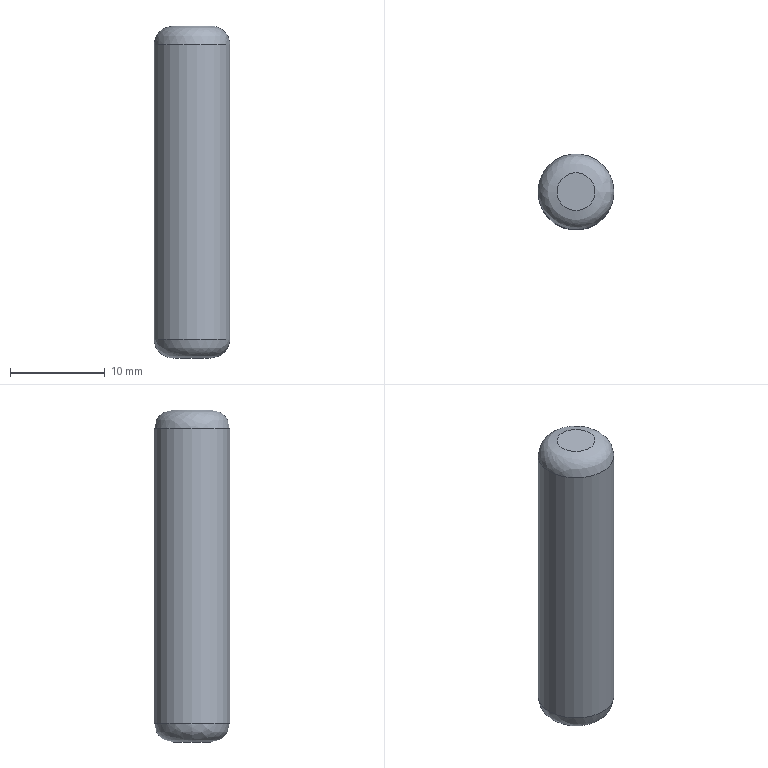Part | STEP file | Tube feed_id1706_x_t | 1 solid | 5 faces | box 8 x 8 x 35 mm | volume 1721 mm3 | plane 2 | spline 2 | cylinder 1 | commonest cylinder face diameters 8 x1
STEP:
#1=CARTESIAN_POINT('',(0.,0.,0.));
#2=DIRECTION('',(0.,0.,1.));
#3=DIRECTION('',(1.,0.,0.));
#4=AXIS2_PLACEMENT_3D('',#1,#2,#3);
#5=CARTESIAN_POINT('',(119.,82.036,-214.5));
#6=VERTEX_POINT('',#5);
#7=CARTESIAN_POINT('',(121.,82.036,-214.5));
#8=DIRECTION('',(0.,0.,-1.));
#9=DIRECTION('',(-1.,0.,0.));
#10=AXIS2_PLACEMENT_3D('',#7,#8,#9);
#11=CIRCLE('',#10,2.);
#12=CARTESIAN_POINT('',(121.,82.036,-214.5));
#13=DIRECTION('',(0.,0.,-1.));
#14=DIRECTION('',(-1.,0.,0.));
#15=AXIS2_PLACEMENT_3D('',#12,#13,#14);
#16=PLANE('',#15);
#17=CARTESIAN_POINT('',(0.,0.));
#18=DIRECTION('',(1.,0.));
#19=AXIS2_PLACEMENT_2D('',#17,#18);
#20=CIRCLE('',#19,2.);
#21=(GEOMETRIC_REPRESENTATION_CONTEXT(2)PARAMETRIC_REPRESENTATION_CONTEXT()REPRESENTATION_CONTEXT('',''));
#22=DEFINITIONAL_REPRESENTATION('',(#20),#21);
#23=PCURVE('',#16,#22);
#24=CARTESIAN_POINT('',(119.,82.036,-214.5));
#25=CARTESIAN_POINT('',(119.,86.036,-214.5));
#26=CARTESIAN_POINT('',(123.,86.036,-214.5));
#27=CARTESIAN_POINT('',(123.,82.036,-214.5));
#28=CARTESIAN_POINT('',(123.,78.036,-214.5));
#29=CARTESIAN_POINT('',(119.,78.036,-214.5));
#30=CARTESIAN_POINT('',(119.,82.036,-214.5));
#31=CARTESIAN_POINT('',(117.828,82.036,-214.5));
#32=CARTESIAN_POINT('',(117.828,88.379,-214.5));
#33=CARTESIAN_POINT('',(124.172,88.379,-214.5));
#34=CARTESIAN_POINT('',(124.172,82.036,-214.5));
#35=CARTESIAN_POINT('',(124.172,75.692,-214.5));
#36=CARTESIAN_POINT('',(117.828,75.692,-214.5));
#37=CARTESIAN_POINT('',(117.828,82.036,-214.5));
#38=CARTESIAN_POINT('',(117.,82.036,-213.672));
#39=CARTESIAN_POINT('',(117.,90.036,-213.672));
#40=CARTESIAN_POINT('',(125.,90.036,-213.672));
#41=CARTESIAN_POINT('',(125.,82.036,-213.672));
#42=CARTESIAN_POINT('',(125.,74.036,-213.672));
#43=CARTESIAN_POINT('',(117.,74.036,-213.672));
#44=CARTESIAN_POINT('',(117.,82.036,-213.672));
#45=CARTESIAN_POINT('',(117.,82.036,-212.5));
#46=CARTESIAN_POINT('',(117.,90.036,-212.5));
#47=CARTESIAN_POINT('',(125.,90.036,-212.5));
#48=CARTESIAN_POINT('',(125.,82.036,-212.5));
#49=CARTESIAN_POINT('',(125.,74.036,-212.5));
#50=CARTESIAN_POINT('',(117.,74.036,-212.5));
#51=CARTESIAN_POINT('',(117.,82.036,-212.5));
#52=(BOUNDED_SURFACE()B_SPLINE_SURFACE(3,3,((#24,#25,#26,#27,#28,#29,#30),(#31,#32,#33,#34,#35,#36,#37),(#38,#39,#40,#41,#42,#43,#44),(#45,#46,#47,#48,#49,#50,#51)),.UNSPECIFIED.,.F.,.T.,.F.)B_SPLINE_SURFACE_WITH_KNOTS((4,4),(1,3,3,3,1),(0.,1.),(-0.5,0.,0.5,1.,1.5),.UNSPECIFIED.)GEOMETRIC_REPRESENTATION_ITEM()RATIONAL_B_SPLINE_SURFACE(((1.,0.3333,0.3333,1.,0.3333,0.3333,1.),(0.8047,0.2682,0.2682,0.8047,0.2682,0.2682,0.8047),(0.8047,0.2682,0.2682,0.8047,0.2682,0.2682,0.8047),(1.,0.3333,0.3333,1.,0.3333,0.3333,1.)))REPRESENTATION_ITEM('')SURFACE());
#53=CARTESIAN_POINT('',(0.,0.));
#54=CARTESIAN_POINT('',(0.,0.02352));
#55=CARTESIAN_POINT('',(0.,0.06491));
#56=CARTESIAN_POINT('',(0.,0.1146));
#57=CARTESIAN_POINT('',(0.,0.1575));
#58=CARTESIAN_POINT('',(0.,0.196));
#59=CARTESIAN_POINT('',(0.,0.2322));
#60=CARTESIAN_POINT('',(0.,0.2678));
#61=CARTESIAN_POINT('',(0.,0.304));
#62=CARTESIAN_POINT('',(0.,0.3425));
#63=CARTESIAN_POINT('',(0.,0.3856));
#64=CARTESIAN_POINT('',(0.,0.4343));
#65=CARTESIAN_POINT('',(0.,0.5));
#66=CARTESIAN_POINT('',(0.,0.5657));
#67=CARTESIAN_POINT('',(0.,0.6144));
#68=CARTESIAN_POINT('',(0.,0.6575));
#69=CARTESIAN_POINT('',(0.,0.696));
#70=CARTESIAN_POINT('',(0.,0.7322));
#71=CARTESIAN_POINT('',(0.,0.7678));
#72=CARTESIAN_POINT('',(0.,0.804));
#73=CARTESIAN_POINT('',(0.,0.8425));
#74=CARTESIAN_POINT('',(0.,0.8854));
#75=CARTESIAN_POINT('',(0.,0.9351));
#76=CARTESIAN_POINT('',(0.,0.9765));
#77=CARTESIAN_POINT('',(0.,1.));
#78=B_SPLINE_CURVE_WITH_KNOTS('',3,(#53,#54,#55,#56,#57,#58,#59,#60,#61,#62,#63,#64,#65,#66,#67,#68,#69,#70,#71,#72,#73,#74,#75,#76,#77),.UNSPECIFIED.,.F.,.F.,(4,1,1,1,1,1,1,1,1,1,1,1,1,1,1,1,1,1,1,1,1,1,4),(0.,0.2856,0.5712,0.8568,1.142,1.428,1.714,1.999,2.285,2.57,2.856,3.142,3.427,3.713,3.998,4.284,4.57,4.855,5.141,5.426,5.712,5.998,6.283),.QUASI_UNIFORM_KNOTS.);
#79=(GEOMETRIC_REPRESENTATION_CONTEXT(2)PARAMETRIC_REPRESENTATION_CONTEXT()REPRESENTATION_CONTEXT('',''));
#80=DEFINITIONAL_REPRESENTATION('',(#78),#79);
#81=PCURVE('',#52,#80);
#82=SURFACE_CURVE('',#11,(#23,#81),.PCURVE_S1.);
#83=EDGE_CURVE('',#6,#6,#82,.T.);
#84=ORIENTED_EDGE('',*,*,#83,.T.);
#85=EDGE_LOOP('',(#84));
#86=FACE_BOUND('',#85,.T.);
#87=ADVANCED_FACE('',(#86),#16,.T.);
#88=CARTESIAN_POINT('',(123.,82.036,-179.5));
#89=VERTEX_POINT('',#88);
#90=CARTESIAN_POINT('',(121.,82.036,-179.5));
#91=DIRECTION('',(0.,0.,1.));
#92=DIRECTION('',(1.,0.,0.));
#93=AXIS2_PLACEMENT_3D('',#90,#91,#92);
#94=CIRCLE('',#93,2.);
#95=CARTESIAN_POINT('',(121.,82.036,-179.5));
#96=DIRECTION('',(0.,0.,1.));
#97=DIRECTION('',(1.,0.,0.));
#98=AXIS2_PLACEMENT_3D('',#95,#96,#97);
#99=PLANE('',#98);
#100=CARTESIAN_POINT('',(0.,0.));
#101=DIRECTION('',(1.,0.));
#102=AXIS2_PLACEMENT_2D('',#100,#101);
#103=CIRCLE('',#102,2.);
#104=(GEOMETRIC_REPRESENTATION_CONTEXT(2)PARAMETRIC_REPRESENTATION_CONTEXT()REPRESENTATION_CONTEXT('',''));
#105=DEFINITIONAL_REPRESENTATION('',(#103),#104);
#106=PCURVE('',#99,#105);
#107=CARTESIAN_POINT('',(123.,82.036,-179.5));
#108=CARTESIAN_POINT('',(123.,86.036,-179.5));
#109=CARTESIAN_POINT('',(119.,86.036,-179.5));
#110=CARTESIAN_POINT('',(119.,82.036,-179.5));
#111=CARTESIAN_POINT('',(119.,78.036,-179.5));
#112=CARTESIAN_POINT('',(123.,78.036,-179.5));
#113=CARTESIAN_POINT('',(123.,82.036,-179.5));
#114=CARTESIAN_POINT('',(124.172,82.036,-179.5));
#115=CARTESIAN_POINT('',(124.172,88.379,-179.5));
#116=CARTESIAN_POINT('',(117.828,88.379,-179.5));
#117=CARTESIAN_POINT('',(117.828,82.036,-179.5));
#118=CARTESIAN_POINT('',(117.828,75.692,-179.5));
#119=CARTESIAN_POINT('',(124.172,75.692,-179.5));
#120=CARTESIAN_POINT('',(124.172,82.036,-179.5));
#121=CARTESIAN_POINT('',(125.,82.036,-180.328));
#122=CARTESIAN_POINT('',(125.,90.036,-180.328));
#123=CARTESIAN_POINT('',(117.,90.036,-180.328));
#124=CARTESIAN_POINT('',(117.,82.036,-180.328));
#125=CARTESIAN_POINT('',(117.,74.036,-180.328));
#126=CARTESIAN_POINT('',(125.,74.036,-180.328));
#127=CARTESIAN_POINT('',(125.,82.036,-180.328));
#128=CARTESIAN_POINT('',(125.,82.036,-181.5));
#129=CARTESIAN_POINT('',(125.,90.036,-181.5));
#130=CARTESIAN_POINT('',(117.,90.036,-181.5));
#131=CARTESIAN_POINT('',(117.,82.036,-181.5));
#132=CARTESIAN_POINT('',(117.,74.036,-181.5));
#133=CARTESIAN_POINT('',(125.,74.036,-181.5));
#134=CARTESIAN_POINT('',(125.,82.036,-181.5));
#135=(BOUNDED_SURFACE()B_SPLINE_SURFACE(3,3,((#107,#108,#109,#110,#111,#112,#113),(#114,#115,#116,#117,#118,#119,#120),(#121,#122,#123,#124,#125,#126,#127),(#128,#129,#130,#131,#132,#133,#134)),.UNSPECIFIED.,.F.,.T.,.F.)B_SPLINE_SURFACE_WITH_KNOTS((4,4),(1,3,3,3,1),(0.,1.),(-0.5,0.,0.5,1.,1.5),.UNSPECIFIED.)GEOMETRIC_REPRESENTATION_ITEM()RATIONAL_B_SPLINE_SURFACE(((1.,0.3333,0.3333,1.,0.3333,0.3333,1.),(0.8047,0.2682,0.2682,0.8047,0.2682,0.2682,0.8047),(0.8047,0.2682,0.2682,0.8047,0.2682,0.2682,0.8047),(1.,0.3333,0.3333,1.,0.3333,0.3333,1.)))REPRESENTATION_ITEM('')SURFACE());
#136=CARTESIAN_POINT('',(0.,0.));
#137=CARTESIAN_POINT('',(0.,0.02352));
#138=CARTESIAN_POINT('',(0.,0.06491));
#139=CARTESIAN_POINT('',(0.,0.1146));
#140=CARTESIAN_POINT('',(0.,0.1575));
#141=CARTESIAN_POINT('',(0.,0.196));
#142=CARTESIAN_POINT('',(0.,0.2322));
#143=CARTESIAN_POINT('',(0.,0.2678));
#144=CARTESIAN_POINT('',(0.,0.304));
#145=CARTESIAN_POINT('',(0.,0.3425));
#146=CARTESIAN_POINT('',(0.,0.3856));
#147=CARTESIAN_POINT('',(0.,0.4343));
#148=CARTESIAN_POINT('',(0.,0.5));
#149=CARTESIAN_POINT('',(0.,0.5657));
#150=CARTESIAN_POINT('',(0.,0.6144));
#151=CARTESIAN_POINT('',(0.,0.6575));
#152=CARTESIAN_POINT('',(0.,0.696));
#153=CARTESIAN_POINT('',(0.,0.7322));
#154=CARTESIAN_POINT('',(0.,0.7678));
#155=CARTESIAN_POINT('',(0.,0.804));
#156=CARTESIAN_POINT('',(0.,0.8425));
#157=CARTESIAN_POINT('',(0.,0.8854));
#158=CARTESIAN_POINT('',(0.,0.9351));
#159=CARTESIAN_POINT('',(0.,0.9765));
#160=CARTESIAN_POINT('',(0.,1.));
#161=B_SPLINE_CURVE_WITH_KNOTS('',3,(#136,#137,#138,#139,#140,#141,#142,#143,#144,#145,#146,#147,#148,#149,#150,#151,#152,#153,#154,#155,#156,#157,#158,#159,#160),.UNSPECIFIED.,.F.,.F.,(4,1,1,1,1,1,1,1,1,1,1,1,1,1,1,1,1,1,1,1,1,1,4),(0.,0.2856,0.5712,0.8568,1.142,1.428,1.714,1.999,2.285,2.57,2.856,3.142,3.427,3.713,3.998,4.284,4.57,4.855,5.141,5.426,5.712,5.998,6.283),.QUASI_UNIFORM_KNOTS.);
#162=(GEOMETRIC_REPRESENTATION_CONTEXT(2)PARAMETRIC_REPRESENTATION_CONTEXT()REPRESENTATION_CONTEXT('',''));
#163=DEFINITIONAL_REPRESENTATION('',(#161),#162);
#164=PCURVE('',#135,#163);
#165=SURFACE_CURVE('',#94,(#106,#164),.PCURVE_S1.);
#166=EDGE_CURVE('',#89,#89,#165,.T.);
#167=ORIENTED_EDGE('',*,*,#166,.T.);
#168=EDGE_LOOP('',(#167));
#169=FACE_BOUND('',#168,.T.);
#170=ADVANCED_FACE('',(#169),#99,.T.);
#171=CARTESIAN_POINT('',(125.,82.036,-181.5));
#172=VERTEX_POINT('',#171);
#173=CARTESIAN_POINT('',(121.,82.036,-181.5));
#174=DIRECTION('',(0.,0.,-1.));
#175=DIRECTION('',(1.,0.,0.));
#176=AXIS2_PLACEMENT_3D('',#173,#174,#175);
#177=CIRCLE('',#176,4.);
#178=CARTESIAN_POINT('',(121.,82.036,-179.5));
#179=DIRECTION('',(0.,0.,-1.));
#180=DIRECTION('',(1.,0.,0.));
#181=AXIS2_PLACEMENT_3D('',#178,#179,#180);
#182=CYLINDRICAL_SURFACE('',#181,4.);
#183=CARTESIAN_POINT('',(0.,2.));
#184=DIRECTION('',(1.,0.));
#185=VECTOR('',#184,1.);
#186=LINE('',#183,#185);
#187=(GEOMETRIC_REPRESENTATION_CONTEXT(2)PARAMETRIC_REPRESENTATION_CONTEXT()REPRESENTATION_CONTEXT('',''));
#188=DEFINITIONAL_REPRESENTATION('',(#186),#187);
#189=PCURVE('',#182,#188);
#190=CARTESIAN_POINT('',(1.,1.));
#191=CARTESIAN_POINT('',(1.,0.9765));
#192=CARTESIAN_POINT('',(1.,0.9351));
#193=CARTESIAN_POINT('',(1.,0.8854));
#194=CARTESIAN_POINT('',(1.,0.8425));
#195=CARTESIAN_POINT('',(1.,0.804));
#196=CARTESIAN_POINT('',(1.,0.7678));
#197=CARTESIAN_POINT('',(1.,0.7322));
#198=CARTESIAN_POINT('',(1.,0.696));
#199=CARTESIAN_POINT('',(1.,0.6575));
#200=CARTESIAN_POINT('',(1.,0.6144));
#201=CARTESIAN_POINT('',(1.,0.5657));
#202=CARTESIAN_POINT('',(1.,0.5));
#203=CARTESIAN_POINT('',(1.,0.4343));
#204=CARTESIAN_POINT('',(1.,0.3856));
#205=CARTESIAN_POINT('',(1.,0.3425));
#206=CARTESIAN_POINT('',(1.,0.304));
#207=CARTESIAN_POINT('',(1.,0.2678));
#208=CARTESIAN_POINT('',(1.,0.2322));
#209=CARTESIAN_POINT('',(1.,0.196));
#210=CARTESIAN_POINT('',(1.,0.1575));
#211=CARTESIAN_POINT('',(1.,0.1146));
#212=CARTESIAN_POINT('',(1.,0.06491));
#213=CARTESIAN_POINT('',(1.,0.02352));
#214=CARTESIAN_POINT('',(1.,0.));
#215=B_SPLINE_CURVE_WITH_KNOTS('',3,(#190,#191,#192,#193,#194,#195,#196,#197,#198,#199,#200,#201,#202,#203,#204,#205,#206,#207,#208,#209,#210,#211,#212,#213,#214),.UNSPECIFIED.,.F.,.F.,(4,1,1,1,1,1,1,1,1,1,1,1,1,1,1,1,1,1,1,1,1,1,4),(0.,0.2856,0.5712,0.8568,1.142,1.428,1.714,1.999,2.285,2.57,2.856,3.142,3.427,3.713,3.998,4.284,4.57,4.855,5.141,5.426,5.712,5.998,6.283),.QUASI_UNIFORM_KNOTS.);
#216=(GEOMETRIC_REPRESENTATION_CONTEXT(2)PARAMETRIC_REPRESENTATION_CONTEXT()REPRESENTATION_CONTEXT('',''));
#217=DEFINITIONAL_REPRESENTATION('',(#215),#216);
#218=PCURVE('',#135,#217);
#219=SURFACE_CURVE('',#177,(#189,#218),.PCURVE_S1.);
#220=EDGE_CURVE('',#172,#172,#219,.T.);
#221=ORIENTED_EDGE('',*,*,#220,.T.);
#222=CARTESIAN_POINT('',(125.,82.036,-212.5));
#223=VERTEX_POINT('',#222);
#224=CARTESIAN_POINT('',(125.,82.036,-181.5));
#225=CARTESIAN_POINT('',(125.,82.036,-212.5));
#226=B_SPLINE_CURVE_WITH_KNOTS('',1,(#224,#225),.UNSPECIFIED.,.F.,.F.,(2,2),(2.,33.),.PIECEWISE_BEZIER_KNOTS.);
#227=CARTESIAN_POINT('',(6.283,0.));
#228=DIRECTION('',(0.,1.));
#229=VECTOR('',#228,1.);
#230=LINE('',#227,#229);
#231=(GEOMETRIC_REPRESENTATION_CONTEXT(2)PARAMETRIC_REPRESENTATION_CONTEXT()REPRESENTATION_CONTEXT('',''));
#232=DEFINITIONAL_REPRESENTATION('',(#230),#231);
#233=PCURVE('',#182,#232);
#234=CARTESIAN_POINT('',(0.,0.));
#235=DIRECTION('',(0.,1.));
#236=VECTOR('',#235,1.);
#237=LINE('',#234,#236);
#238=(GEOMETRIC_REPRESENTATION_CONTEXT(2)PARAMETRIC_REPRESENTATION_CONTEXT()REPRESENTATION_CONTEXT('',''));
#239=DEFINITIONAL_REPRESENTATION('',(#237),#238);
#240=PCURVE('',#182,#239);
#241=SEAM_CURVE('',#226,(#233,#240),.PCURVE_S1.);
#242=EDGE_CURVE('',#172,#223,#241,.T.);
#243=ORIENTED_EDGE('',*,*,#242,.T.);
#244=CARTESIAN_POINT('',(117.,82.036,-212.5));
#245=VERTEX_POINT('',#244);
#246=CARTESIAN_POINT('',(121.,82.036,-212.5));
#247=DIRECTION('',(0.,0.,1.));
#248=DIRECTION('',(-1.,0.,0.));
#249=AXIS2_PLACEMENT_3D('',#246,#247,#248);
#250=CIRCLE('',#249,4.);
#251=CARTESIAN_POINT('',(9.425,33.));
#252=DIRECTION('',(-1.,0.));
#253=VECTOR('',#252,1.);
#254=LINE('',#251,#253);
#255=(GEOMETRIC_REPRESENTATION_CONTEXT(2)PARAMETRIC_REPRESENTATION_CONTEXT()REPRESENTATION_CONTEXT('',''));
#256=DEFINITIONAL_REPRESENTATION('',(#254),#255);
#257=PCURVE('',#182,#256);
#258=CARTESIAN_POINT('',(1.,0.5));
#259=CARTESIAN_POINT('',(1.,0.4881));
#260=CARTESIAN_POINT('',(1.,0.466));
#261=CARTESIAN_POINT('',(1.,0.4367));
#262=CARTESIAN_POINT('',(1.,0.4103));
#263=CARTESIAN_POINT('',(1.,0.3862));
#264=CARTESIAN_POINT('',(1.,0.3639));
#265=CARTESIAN_POINT('',(1.,0.3431));
#266=CARTESIAN_POINT('',(1.,0.3233));
#267=CARTESIAN_POINT('',(1.,0.3043));
#268=CARTESIAN_POINT('',(1.,0.2859));
#269=CARTESIAN_POINT('',(1.,0.2678));
#270=CARTESIAN_POINT('',(1.,0.25));
#271=CARTESIAN_POINT('',(1.,0.2322));
#272=CARTESIAN_POINT('',(1.,0.2141));
#273=CARTESIAN_POINT('',(1.,0.1957));
#274=CARTESIAN_POINT('',(1.,0.1767));
#275=CARTESIAN_POINT('',(1.,0.1569));
#276=CARTESIAN_POINT('',(1.,0.1361));
#277=CARTESIAN_POINT('',(1.,0.1138));
#278=CARTESIAN_POINT('',(1.,0.08972));
#279=CARTESIAN_POINT('',(1.,0.06334));
#280=CARTESIAN_POINT('',(1.,0.03403));
#281=CARTESIAN_POINT('',(1.,0.01187));
#282=CARTESIAN_POINT('',(1.,0.));
#283=B_SPLINE_CURVE_WITH_KNOTS('',3,(#258,#259,#260,#261,#262,#263,#264,#265,#266,#267,#268,#269,#270,#271,#272,#273,#274,#275,#276,#277,#278,#279,#280,#281,#282),.UNSPECIFIED.,.F.,.F.,(4,1,1,1,1,1,1,1,1,1,1,1,1,1,1,1,1,1,1,1,1,1,4),(3.142,3.284,3.427,3.57,3.713,3.856,3.998,4.141,4.284,4.427,4.57,4.712,4.855,4.998,5.141,5.284,5.426,5.569,5.712,5.855,5.998,6.14,6.283),.QUASI_UNIFORM_KNOTS.);
#284=(GEOMETRIC_REPRESENTATION_CONTEXT(2)PARAMETRIC_REPRESENTATION_CONTEXT()REPRESENTATION_CONTEXT('',''));
#285=DEFINITIONAL_REPRESENTATION('',(#283),#284);
#286=PCURVE('',#52,#285);
#287=SURFACE_CURVE('',#250,(#257,#286),.PCURVE_S1.);
#288=EDGE_CURVE('',#223,#245,#287,.T.);
#289=ORIENTED_EDGE('',*,*,#288,.T.);
#290=CARTESIAN_POINT('',(121.,82.036,-212.5));
#291=DIRECTION('',(0.,0.,1.));
#292=DIRECTION('',(-1.,0.,0.));
#293=AXIS2_PLACEMENT_3D('',#290,#291,#292);
#294=CIRCLE('',#293,4.);
#295=CARTESIAN_POINT('',(3.142,33.));
#296=DIRECTION('',(-1.,0.));
#297=VECTOR('',#296,1.);
#298=LINE('',#295,#297);
#299=(GEOMETRIC_REPRESENTATION_CONTEXT(2)PARAMETRIC_REPRESENTATION_CONTEXT()REPRESENTATION_CONTEXT('',''));
#300=DEFINITIONAL_REPRESENTATION('',(#298),#299);
#301=PCURVE('',#182,#300);
#302=CARTESIAN_POINT('',(1.,1.));
#303=CARTESIAN_POINT('',(1.,0.9881));
#304=CARTESIAN_POINT('',(1.,0.966));
#305=CARTESIAN_POINT('',(1.,0.9367));
#306=CARTESIAN_POINT('',(1.,0.9103));
#307=CARTESIAN_POINT('',(1.,0.8862));
#308=CARTESIAN_POINT('',(1.,0.8639));
#309=CARTESIAN_POINT('',(1.,0.8431));
#310=CARTESIAN_POINT('',(1.,0.8233));
#311=CARTESIAN_POINT('',(1.,0.8043));
#312=CARTESIAN_POINT('',(1.,0.7859));
#313=CARTESIAN_POINT('',(1.,0.7678));
#314=CARTESIAN_POINT('',(1.,0.75));
#315=CARTESIAN_POINT('',(1.,0.7322));
#316=CARTESIAN_POINT('',(1.,0.7141));
#317=CARTESIAN_POINT('',(1.,0.6957));
#318=CARTESIAN_POINT('',(1.,0.6767));
#319=CARTESIAN_POINT('',(1.,0.6569));
#320=CARTESIAN_POINT('',(1.,0.6361));
#321=CARTESIAN_POINT('',(1.,0.6138));
#322=CARTESIAN_POINT('',(1.,0.5897));
#323=CARTESIAN_POINT('',(1.,0.5633));
#324=CARTESIAN_POINT('',(1.,0.534));
#325=CARTESIAN_POINT('',(1.,0.5119));
#326=CARTESIAN_POINT('',(1.,0.5));
#327=B_SPLINE_CURVE_WITH_KNOTS('',3,(#302,#303,#304,#305,#306,#307,#308,#309,#310,#311,#312,#313,#314,#315,#316,#317,#318,#319,#320,#321,#322,#323,#324,#325,#326),.UNSPECIFIED.,.F.,.F.,(4,1,1,1,1,1,1,1,1,1,1,1,1,1,1,1,1,1,1,1,1,1,4),(0.,0.1428,0.2856,0.4284,0.5712,0.714,0.8568,0.9996,1.142,1.285,1.428,1.571,1.714,1.856,1.999,2.142,2.285,2.428,2.57,2.713,2.856,2.999,3.142),.QUASI_UNIFORM_KNOTS.);
#328=(GEOMETRIC_REPRESENTATION_CONTEXT(2)PARAMETRIC_REPRESENTATION_CONTEXT()REPRESENTATION_CONTEXT('',''));
#329=DEFINITIONAL_REPRESENTATION('',(#327),#328);
#330=PCURVE('',#52,#329);
#331=SURFACE_CURVE('',#294,(#301,#330),.PCURVE_S1.);
#332=EDGE_CURVE('',#245,#223,#331,.T.);
#333=ORIENTED_EDGE('',*,*,#332,.T.);
#334=ORIENTED_EDGE('',*,*,#242,.F.);
#335=EDGE_LOOP('',(#221,#243,#289,#333,#334));
#336=FACE_BOUND('',#335,.T.);
#337=ADVANCED_FACE('',(#336),#182,.T.);
#338=ORIENTED_EDGE('',*,*,#166,.F.);
#339=CARTESIAN_POINT('',(123.,82.036,-179.5));
#340=CARTESIAN_POINT('',(124.172,82.036,-179.5));
#341=CARTESIAN_POINT('',(125.,82.036,-180.328));
#342=CARTESIAN_POINT('',(125.,82.036,-181.5));
#343=(BOUNDED_CURVE()B_SPLINE_CURVE(3,(#339,#340,#341,#342),.UNSPECIFIED.,.F.,.F.)B_SPLINE_CURVE_WITH_KNOTS((4,4),(0.,1.),.PIECEWISE_BEZIER_KNOTS.)CURVE()GEOMETRIC_REPRESENTATION_ITEM()RATIONAL_B_SPLINE_CURVE((1.,0.8047,0.8047,1.))REPRESENTATION_ITEM(''));
#344=CARTESIAN_POINT('',(0.,0.));
#345=DIRECTION('',(1.,0.));
#346=VECTOR('',#345,1.);
#347=LINE('',#344,#346);
#348=(GEOMETRIC_REPRESENTATION_CONTEXT(2)PARAMETRIC_REPRESENTATION_CONTEXT()REPRESENTATION_CONTEXT('',''));
#349=DEFINITIONAL_REPRESENTATION('',(#347),#348);
#350=PCURVE('',#135,#349);
#351=CARTESIAN_POINT('',(0.,1.));
#352=DIRECTION('',(1.,0.));
#353=VECTOR('',#352,1.);
#354=LINE('',#351,#353);
#355=(GEOMETRIC_REPRESENTATION_CONTEXT(2)PARAMETRIC_REPRESENTATION_CONTEXT()REPRESENTATION_CONTEXT('',''));
#356=DEFINITIONAL_REPRESENTATION('',(#354),#355);
#357=PCURVE('',#135,#356);
#358=SEAM_CURVE('',#343,(#350,#357),.PCURVE_S1.);
#359=EDGE_CURVE('',#89,#172,#358,.T.);
#360=ORIENTED_EDGE('',*,*,#359,.T.);
#361=ORIENTED_EDGE('',*,*,#220,.F.);
#362=ORIENTED_EDGE('',*,*,#359,.F.);
#363=EDGE_LOOP('',(#338,#360,#361,#362));
#364=FACE_BOUND('',#363,.T.);
#365=ADVANCED_FACE('',(#364),#135,.T.);
#366=ORIENTED_EDGE('',*,*,#83,.F.);
#367=CARTESIAN_POINT('',(119.,82.036,-214.5));
#368=CARTESIAN_POINT('',(117.828,82.036,-214.5));
#369=CARTESIAN_POINT('',(117.,82.036,-213.672));
#370=CARTESIAN_POINT('',(117.,82.036,-212.5));
#371=(BOUNDED_CURVE()B_SPLINE_CURVE(3,(#367,#368,#369,#370),.UNSPECIFIED.,.F.,.F.)B_SPLINE_CURVE_WITH_KNOTS((4,4),(0.,1.),.PIECEWISE_BEZIER_KNOTS.)CURVE()GEOMETRIC_REPRESENTATION_ITEM()RATIONAL_B_SPLINE_CURVE((1.,0.8047,0.8047,1.))REPRESENTATION_ITEM(''));
#372=CARTESIAN_POINT('',(0.,0.));
#373=DIRECTION('',(1.,0.));
#374=VECTOR('',#373,1.);
#375=LINE('',#372,#374);
#376=(GEOMETRIC_REPRESENTATION_CONTEXT(2)PARAMETRIC_REPRESENTATION_CONTEXT()REPRESENTATION_CONTEXT('',''));
#377=DEFINITIONAL_REPRESENTATION('',(#375),#376);
#378=PCURVE('',#52,#377);
#379=CARTESIAN_POINT('',(0.,1.));
#380=DIRECTION('',(1.,0.));
#381=VECTOR('',#380,1.);
#382=LINE('',#379,#381);
#383=(GEOMETRIC_REPRESENTATION_CONTEXT(2)PARAMETRIC_REPRESENTATION_CONTEXT()REPRESENTATION_CONTEXT('',''));
#384=DEFINITIONAL_REPRESENTATION('',(#382),#383);
#385=PCURVE('',#52,#384);
#386=SEAM_CURVE('',#371,(#378,#385),.PCURVE_S1.);
#387=EDGE_CURVE('',#6,#245,#386,.T.);
#388=ORIENTED_EDGE('',*,*,#387,.T.);
#389=ORIENTED_EDGE('',*,*,#288,.F.);
#390=ORIENTED_EDGE('',*,*,#332,.F.);
#391=ORIENTED_EDGE('',*,*,#387,.F.);
#392=EDGE_LOOP('',(#366,#388,#389,#390,#391));
#393=FACE_BOUND('',#392,.T.);
#394=ADVANCED_FACE('',(#393),#52,.T.);
#395=CLOSED_SHELL('',(#87,#170,#337,#365,#394));
#396=MANIFOLD_SOLID_BREP('',#395);
#397=(LENGTH_UNIT()NAMED_UNIT(*)SI_UNIT(.MILLI.,.METRE.));
#398=UNCERTAINTY_MEASURE_WITH_UNIT(LENGTH_MEASURE(0.00001),#397,'','');
#399=(NAMED_UNIT(*)PLANE_ANGLE_UNIT()SI_UNIT($,.RADIAN.));
#400=(NAMED_UNIT(*)SI_UNIT($,.STERADIAN.)SOLID_ANGLE_UNIT());
#401=(GEOMETRIC_REPRESENTATION_CONTEXT(3)GLOBAL_UNCERTAINTY_ASSIGNED_CONTEXT((#398))GLOBAL_UNIT_ASSIGNED_CONTEXT((#397,#399,#400))REPRESENTATION_CONTEXT('',''));
#402=ADVANCED_BREP_SHAPE_REPRESENTATION('',(#4,#396),#401);